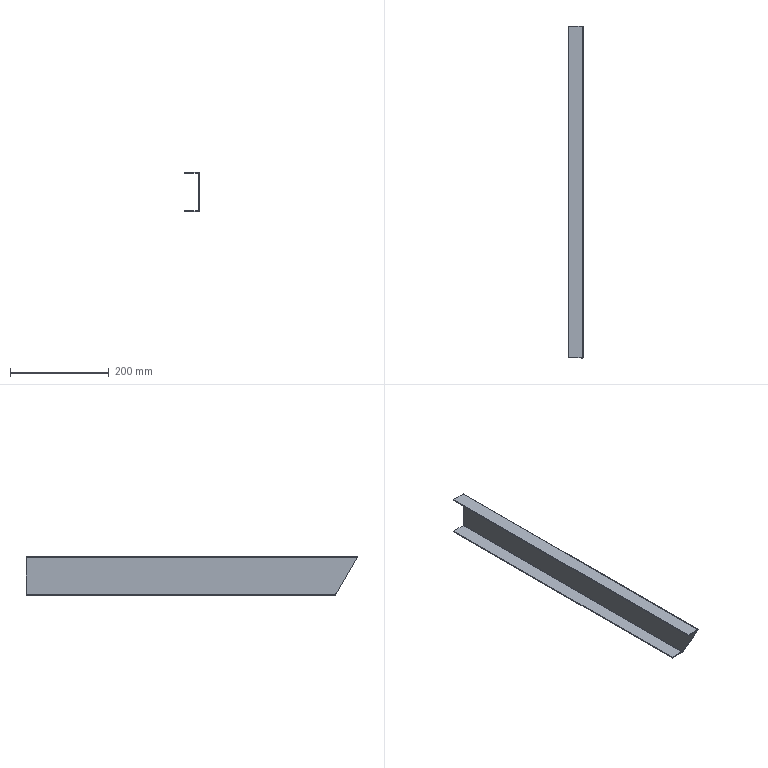Part | STEP file | Guard Rib | 1 solid | 19 faces | box 30 x 673.333 x 80 mm | volume 175185 mm3 | plane 13 | cylinder 5 | spline 1 | commonest cylinder face diameters 1 x3 5 x2
STEP:
#1=CARTESIAN_POINT('',(0.,265.398,-132.691));
#2=VERTEX_POINT('',#1);
#3=CARTESIAN_POINT('',(0.,221.653,-56.923));
#4=VERTEX_POINT('',#3);
#5=CARTESIAN_POINT('',(0.,265.398,-132.691));
#6=DIRECTION('',(0.,-0.5,0.866));
#7=VECTOR('',#6,1000.);
#8=LINE('',#5,#7);
#9=EDGE_CURVE('',#2,#4,#8,.T.);
#10=ORIENTED_EDGE('',*,*,#9,.F.);
#11=CARTESIAN_POINT('',(0.,265.398,-130.923));
#12=VERTEX_POINT('',#11);
#13=CARTESIAN_POINT('',(0.,265.398,0.));
#14=DIRECTION('',(0.,0.,-1.));
#15=VECTOR('',#14,1000.);
#16=LINE('',#13,#15);
#17=EDGE_CURVE('',#12,#2,#16,.T.);
#18=ORIENTED_EDGE('',*,*,#17,.F.);
#19=CARTESIAN_POINT('',(0.,266.398,-130.923));
#20=VERTEX_POINT('',#19);
#21=CARTESIAN_POINT('',(0.,265.898,-130.923));
#22=DIRECTION('',(-1.,0.,0.));
#23=DIRECTION('',(0.,0.,-1.));
#24=AXIS2_PLACEMENT_3D('',#21,#22,#23);
#25=CIRCLE('',#24,0.5);
#26=EDGE_CURVE('',#12,#20,#25,.T.);
#27=ORIENTED_EDGE('',*,*,#26,.T.);
#28=CARTESIAN_POINT('',(0.,266.398,-131.923));
#29=VERTEX_POINT('',#28);
#30=CARTESIAN_POINT('',(0.,266.398,-130.923));
#31=DIRECTION('',(0.,0.,1.));
#32=VECTOR('',#31,1000.);
#33=LINE('',#30,#32);
#34=EDGE_CURVE('',#29,#20,#33,.T.);
#35=ORIENTED_EDGE('',*,*,#34,.F.);
#36=CARTESIAN_POINT('',(0.,893.543,-131.923));
#37=VERTEX_POINT('',#36);
#38=CARTESIAN_POINT('',(0.,0.,-131.923));
#39=DIRECTION('',(0.,-1.,0.));
#40=VECTOR('',#39,1000.);
#41=LINE('',#38,#40);
#42=EDGE_CURVE('',#37,#29,#41,.T.);
#43=ORIENTED_EDGE('',*,*,#42,.F.);
#44=CARTESIAN_POINT('',(0.,893.543,-56.923));
#45=VERTEX_POINT('',#44);
#46=CARTESIAN_POINT('',(0.,893.543,0.));
#47=DIRECTION('',(0.,0.,-1.));
#48=VECTOR('',#47,1000.);
#49=LINE('',#46,#48);
#50=EDGE_CURVE('',#45,#37,#49,.T.);
#51=ORIENTED_EDGE('',*,*,#50,.F.);
#52=CARTESIAN_POINT('',(0.,0.,-56.923));
#53=DIRECTION('',(0.,1.,0.));
#54=VECTOR('',#53,1000.);
#55=LINE('',#52,#54);
#56=EDGE_CURVE('',#4,#45,#55,.T.);
#57=ORIENTED_EDGE('',*,*,#56,.F.);
#58=EDGE_LOOP('',(#10,#18,#27,#35,#43,#51,#57));
#59=FACE_OUTER_BOUND('',#58,.T.);
#60=CARTESIAN_POINT('',(0.,0.,0.));
#61=DIRECTION('',(-1.,0.,0.));
#62=DIRECTION('',(0.,0.,1.));
#63=AXIS2_PLACEMENT_3D('',#60,#61,#62);
#64=PLANE('',#63);
#65=ADVANCED_FACE('',(#59),#64,.F.);
#66=CARTESIAN_POINT('',(-2.5,893.543,-54.423));
#67=VERTEX_POINT('',#66);
#68=CARTESIAN_POINT('',(-2.5,220.21,-54.423));
#69=VERTEX_POINT('',#68);
#70=CARTESIAN_POINT('',(-2.5,893.543,-54.423));
#71=DIRECTION('',(0.,-1.,0.));
#72=VECTOR('',#71,1000.);
#73=LINE('',#70,#72);
#74=EDGE_CURVE('',#67,#69,#73,.T.);
#75=ORIENTED_EDGE('',*,*,#74,.T.);
#76=CARTESIAN_POINT('',(-2.5,220.21,-54.423));
#77=CARTESIAN_POINT('',(-2.17,220.332,-54.423));
#78=CARTESIAN_POINT('',(-1.85,220.449,-54.487));
#79=CARTESIAN_POINT('',(-1.393,220.631,-54.676));
#80=CARTESIAN_POINT('',(-1.248,220.691,-54.753));
#81=CARTESIAN_POINT('',(-0.9774,220.81,-54.934));
#82=CARTESIAN_POINT('',(-0.8497,220.871,-55.038));
#83=CARTESIAN_POINT('',(-0.6169,220.992,-55.271));
#84=CARTESIAN_POINT('',(-0.5135,221.051,-55.397));
#85=CARTESIAN_POINT('',(-0.3321,221.171,-55.668));
#86=CARTESIAN_POINT('',(-0.2536,221.232,-55.814));
#87=CARTESIAN_POINT('',(-0.128,221.352,-56.117));
#88=CARTESIAN_POINT('',(-0.08064,221.412,-56.273));
#89=CARTESIAN_POINT('',(-0.01656,221.532,-56.593));
#90=CARTESIAN_POINT('',(0.,221.593,-56.758));
#91=CARTESIAN_POINT('',(0.,221.653,-56.923));
#92=B_SPLINE_CURVE_WITH_KNOTS('',3,(#76,#77,#78,#79,#80,#81,#82,#83,#84,#85,#86,#87,#88,#89,#90,#91),.UNSPECIFIED.,.F.,.F.,(4,2,2,2,2,2,2,4),(0.,0.001038,0.001557,0.002076,0.002595,0.003114,0.003633,0.004151),.UNSPECIFIED.);
#93=EDGE_CURVE('',#69,#4,#92,.T.);
#94=ORIENTED_EDGE('',*,*,#93,.T.);
#95=ORIENTED_EDGE('',*,*,#56,.T.);
#96=CARTESIAN_POINT('',(-2.5,893.543,-56.923));
#97=DIRECTION('',(0.,-1.,0.));
#98=DIRECTION('',(0.,0.,1.));
#99=AXIS2_PLACEMENT_3D('',#96,#97,#98);
#100=CIRCLE('',#99,2.5);
#101=EDGE_CURVE('',#45,#67,#100,.T.);
#102=ORIENTED_EDGE('',*,*,#101,.T.);
#103=EDGE_LOOP('',(#75,#94,#95,#102));
#104=FACE_OUTER_BOUND('',#103,.T.);
#105=CARTESIAN_POINT('',(-2.5,893.543,-56.923));
#106=DIRECTION('',(0.,1.,0.));
#107=DIRECTION('',(0.,0.,1.));
#108=AXIS2_PLACEMENT_3D('',#105,#106,#107);
#109=CYLINDRICAL_SURFACE('',#108,2.5);
#110=ADVANCED_FACE('',(#104),#109,.T.);
#111=CARTESIAN_POINT('',(-2.,221.653,-56.923));
#112=VERTEX_POINT('',#111);
#113=CARTESIAN_POINT('',(-2.,265.398,-132.691));
#114=VERTEX_POINT('',#113);
#115=CARTESIAN_POINT('',(-2.,220.21,-54.423));
#116=DIRECTION('',(0.,0.5,-0.866));
#117=VECTOR('',#116,1000.);
#118=LINE('',#115,#117);
#119=EDGE_CURVE('',#112,#114,#118,.T.);
#120=ORIENTED_EDGE('',*,*,#119,.T.);
#121=CARTESIAN_POINT('',(-2.,265.398,-132.691));
#122=DIRECTION('',(1.,0.,0.));
#123=VECTOR('',#122,1000.);
#124=LINE('',#121,#123);
#125=EDGE_CURVE('',#114,#2,#124,.T.);
#126=ORIENTED_EDGE('',*,*,#125,.T.);
#127=ORIENTED_EDGE('',*,*,#9,.T.);
#128=CARTESIAN_POINT('',(-2.,221.653,-56.923));
#129=DIRECTION('',(-1.,0.,0.));
#130=VECTOR('',#129,1000.);
#131=LINE('',#128,#130);
#132=EDGE_CURVE('',#4,#112,#131,.T.);
#133=ORIENTED_EDGE('',*,*,#132,.T.);
#134=EDGE_LOOP('',(#120,#126,#127,#133));
#135=FACE_OUTER_BOUND('',#134,.T.);
#136=CARTESIAN_POINT('',(-2.,220.21,-54.423));
#137=DIRECTION('',(0.,-0.866,-0.5));
#138=DIRECTION('',(0.,0.5,-0.866));
#139=AXIS2_PLACEMENT_3D('',#136,#137,#138);
#140=PLANE('',#139);
#141=ADVANCED_FACE('',(#135),#140,.T.);
#142=ORIENTED_EDGE('',*,*,#125,.F.);
#143=CARTESIAN_POINT('',(-2.,265.398,-130.923));
#144=VERTEX_POINT('',#143);
#145=CARTESIAN_POINT('',(-2.,265.398,-132.691));
#146=DIRECTION('',(0.,0.,1.));
#147=VECTOR('',#146,1000.);
#148=LINE('',#145,#147);
#149=EDGE_CURVE('',#114,#144,#148,.T.);
#150=ORIENTED_EDGE('',*,*,#149,.T.);
#151=CARTESIAN_POINT('',(-2.,265.398,-130.923));
#152=DIRECTION('',(1.,0.,0.));
#153=VECTOR('',#152,1000.);
#154=LINE('',#151,#153);
#155=EDGE_CURVE('',#144,#12,#154,.T.);
#156=ORIENTED_EDGE('',*,*,#155,.T.);
#157=ORIENTED_EDGE('',*,*,#17,.T.);
#158=EDGE_LOOP('',(#142,#150,#156,#157));
#159=FACE_OUTER_BOUND('',#158,.T.);
#160=CARTESIAN_POINT('',(-2.,265.398,-132.691));
#161=DIRECTION('',(0.,1.,0.));
#162=DIRECTION('',(0.,0.,1.));
#163=AXIS2_PLACEMENT_3D('',#160,#161,#162);
#164=PLANE('',#163);
#165=ADVANCED_FACE('',(#159),#164,.T.);
#166=CARTESIAN_POINT('',(-2.5,266.398,-134.423));
#167=VERTEX_POINT('',#166);
#168=CARTESIAN_POINT('',(-2.5,893.543,-134.423));
#169=VERTEX_POINT('',#168);
#170=CARTESIAN_POINT('',(-2.5,266.398,-134.423));
#171=DIRECTION('',(0.,1.,0.));
#172=VECTOR('',#171,1000.);
#173=LINE('',#170,#172);
#174=EDGE_CURVE('',#167,#169,#173,.T.);
#175=ORIENTED_EDGE('',*,*,#174,.T.);
#176=CARTESIAN_POINT('',(-2.5,893.543,-131.923));
#177=DIRECTION('',(0.,-1.,0.));
#178=DIRECTION('',(0.,0.,-1.));
#179=AXIS2_PLACEMENT_3D('',#176,#177,#178);
#180=CIRCLE('',#179,2.5);
#181=EDGE_CURVE('',#169,#37,#180,.T.);
#182=ORIENTED_EDGE('',*,*,#181,.T.);
#183=ORIENTED_EDGE('',*,*,#42,.T.);
#184=CARTESIAN_POINT('',(-2.5,266.398,-131.923));
#185=DIRECTION('',(0.,1.,0.));
#186=DIRECTION('',(0.,0.,-1.));
#187=AXIS2_PLACEMENT_3D('',#184,#185,#186);
#188=CIRCLE('',#187,2.5);
#189=EDGE_CURVE('',#29,#167,#188,.T.);
#190=ORIENTED_EDGE('',*,*,#189,.T.);
#191=EDGE_LOOP('',(#175,#182,#183,#190));
#192=FACE_OUTER_BOUND('',#191,.T.);
#193=CARTESIAN_POINT('',(-2.5,266.398,-131.923));
#194=DIRECTION('',(0.,-1.,0.));
#195=DIRECTION('',(0.,0.,-1.));
#196=AXIS2_PLACEMENT_3D('',#193,#194,#195);
#197=CYLINDRICAL_SURFACE('',#196,2.5);
#198=ADVANCED_FACE('',(#192),#197,.T.);
#199=ORIENTED_EDGE('',*,*,#50,.T.);
#200=ORIENTED_EDGE('',*,*,#181,.F.);
#201=CARTESIAN_POINT('',(-30.,893.543,-134.423));
#202=VERTEX_POINT('',#201);
#203=CARTESIAN_POINT('',(0.,893.543,-134.423));
#204=DIRECTION('',(1.,0.,0.));
#205=VECTOR('',#204,1000.);
#206=LINE('',#203,#205);
#207=EDGE_CURVE('',#202,#169,#206,.T.);
#208=ORIENTED_EDGE('',*,*,#207,.F.);
#209=CARTESIAN_POINT('',(-30.,893.543,-132.423));
#210=VERTEX_POINT('',#209);
#211=CARTESIAN_POINT('',(-30.,893.543,-134.423));
#212=DIRECTION('',(0.,0.,1.));
#213=VECTOR('',#212,1000.);
#214=LINE('',#211,#213);
#215=EDGE_CURVE('',#202,#210,#214,.T.);
#216=ORIENTED_EDGE('',*,*,#215,.T.);
#217=CARTESIAN_POINT('',(-2.5,893.543,-132.423));
#218=VERTEX_POINT('',#217);
#219=CARTESIAN_POINT('',(-30.,893.543,-132.423));
#220=DIRECTION('',(1.,0.,0.));
#221=VECTOR('',#220,1000.);
#222=LINE('',#219,#221);
#223=EDGE_CURVE('',#210,#218,#222,.T.);
#224=ORIENTED_EDGE('',*,*,#223,.T.);
#225=CARTESIAN_POINT('',(-2.,893.543,-131.923));
#226=VERTEX_POINT('',#225);
#227=CARTESIAN_POINT('',(-2.5,893.543,-131.923));
#228=DIRECTION('',(0.,-1.,0.));
#229=DIRECTION('',(0.,0.,-1.));
#230=AXIS2_PLACEMENT_3D('',#227,#228,#229);
#231=CIRCLE('',#230,0.5);
#232=EDGE_CURVE('',#218,#226,#231,.T.);
#233=ORIENTED_EDGE('',*,*,#232,.T.);
#234=CARTESIAN_POINT('',(-2.,893.543,-56.923));
#235=VERTEX_POINT('',#234);
#236=CARTESIAN_POINT('',(-2.,893.543,-54.423));
#237=DIRECTION('',(0.,0.,1.));
#238=VECTOR('',#237,1000.);
#239=LINE('',#236,#238);
#240=EDGE_CURVE('',#226,#235,#239,.T.);
#241=ORIENTED_EDGE('',*,*,#240,.T.);
#242=CARTESIAN_POINT('',(-2.5,893.543,-56.423));
#243=VERTEX_POINT('',#242);
#244=CARTESIAN_POINT('',(-2.5,893.543,-56.923));
#245=DIRECTION('',(0.,-1.,0.));
#246=DIRECTION('',(0.,0.,1.));
#247=AXIS2_PLACEMENT_3D('',#244,#245,#246);
#248=CIRCLE('',#247,0.5);
#249=EDGE_CURVE('',#235,#243,#248,.T.);
#250=ORIENTED_EDGE('',*,*,#249,.T.);
#251=CARTESIAN_POINT('',(-30.,893.543,-56.423));
#252=VERTEX_POINT('',#251);
#253=CARTESIAN_POINT('',(-30.,893.543,-56.423));
#254=DIRECTION('',(-1.,0.,0.));
#255=VECTOR('',#254,1000.);
#256=LINE('',#253,#255);
#257=EDGE_CURVE('',#243,#252,#256,.T.);
#258=ORIENTED_EDGE('',*,*,#257,.T.);
#259=CARTESIAN_POINT('',(-30.,893.543,-54.423));
#260=VERTEX_POINT('',#259);
#261=CARTESIAN_POINT('',(-30.,893.543,-54.423));
#262=DIRECTION('',(0.,0.,1.));
#263=VECTOR('',#262,1000.);
#264=LINE('',#261,#263);
#265=EDGE_CURVE('',#252,#260,#264,.T.);
#266=ORIENTED_EDGE('',*,*,#265,.T.);
#267=CARTESIAN_POINT('',(0.,893.543,-54.423));
#268=DIRECTION('',(1.,0.,0.));
#269=VECTOR('',#268,1000.);
#270=LINE('',#267,#269);
#271=EDGE_CURVE('',#260,#67,#270,.T.);
#272=ORIENTED_EDGE('',*,*,#271,.T.);
#273=ORIENTED_EDGE('',*,*,#101,.F.);
#274=EDGE_LOOP('',(#199,#200,#208,#216,#224,#233,#241,#250,#258,#266,#272,#273));
#275=FACE_OUTER_BOUND('',#274,.T.);
#276=CARTESIAN_POINT('',(-2.,893.543,-54.423));
#277=DIRECTION('',(0.,1.,0.));
#278=DIRECTION('',(0.,0.,1.));
#279=AXIS2_PLACEMENT_3D('',#276,#277,#278);
#280=PLANE('',#279);
#281=ADVANCED_FACE('',(#275),#280,.T.);
#282=CARTESIAN_POINT('',(-2.5,220.21,-56.423));
#283=VERTEX_POINT('',#282);
#284=CARTESIAN_POINT('',(-2.5,220.21,-56.423));
#285=CARTESIAN_POINT('',(-2.434,220.331,-56.423));
#286=CARTESIAN_POINT('',(-2.369,220.451,-56.436));
#287=CARTESIAN_POINT('',(-2.249,220.69,-56.486));
#288=CARTESIAN_POINT('',(-2.193,220.811,-56.523));
#289=CARTESIAN_POINT('',(-2.054,221.173,-56.662));
#290=CARTESIAN_POINT('',(-2.,221.411,-56.791));
#291=CARTESIAN_POINT('',(-2.,221.653,-56.923));
#292=B_SPLINE_CURVE_WITH_KNOTS('',3,(#284,#285,#286,#287,#288,#289,#290,#291),.UNSPECIFIED.,.F.,.F.,(4,2,2,4),(0.,0.0004085,0.0008171,0.001634),.UNSPECIFIED.);
#293=EDGE_CURVE('',#283,#112,#292,.T.);
#294=ORIENTED_EDGE('',*,*,#293,.T.);
#295=ORIENTED_EDGE('',*,*,#132,.F.);
#296=ORIENTED_EDGE('',*,*,#93,.F.);
#297=CARTESIAN_POINT('',(-2.5,220.21,-55.423));
#298=DIRECTION('',(0.,0.,1.));
#299=VECTOR('',#298,1000.);
#300=LINE('',#297,#299);
#301=EDGE_CURVE('',#283,#69,#300,.T.);
#302=ORIENTED_EDGE('',*,*,#301,.F.);
#303=EDGE_LOOP('',(#294,#295,#296,#302));
#304=FACE_OUTER_BOUND('',#303,.T.);
#305=CARTESIAN_POINT('',(0.02,221.653,-56.923));
#306=CARTESIAN_POINT('',(0.02,221.533,-56.593));
#307=CARTESIAN_POINT('',(-0.04559,221.413,-56.264));
#308=CARTESIAN_POINT('',(-0.2981,221.172,-55.654));
#309=CARTESIAN_POINT('',(-0.4848,221.052,-55.375));
#310=CARTESIAN_POINT('',(-0.9513,220.812,-54.908));
#311=CARTESIAN_POINT('',(-1.231,220.691,-54.721));
#312=CARTESIAN_POINT('',(-1.84,220.451,-54.469));
#313=CARTESIAN_POINT('',(-2.17,220.33,-54.403));
#314=CARTESIAN_POINT('',(-2.5,220.21,-54.403));
#315=CARTESIAN_POINT('',(0.,221.653,-56.923));
#316=CARTESIAN_POINT('',(0.,221.533,-56.596));
#317=CARTESIAN_POINT('',(-0.06507,221.413,-56.269));
#318=CARTESIAN_POINT('',(-0.3155,221.172,-55.664));
#319=CARTESIAN_POINT('',(-0.5008,221.052,-55.387));
#320=CARTESIAN_POINT('',(-0.9636,220.812,-54.924));
#321=CARTESIAN_POINT('',(-1.241,220.691,-54.739));
#322=CARTESIAN_POINT('',(-1.846,220.451,-54.488));
#323=CARTESIAN_POINT('',(-2.173,220.33,-54.423));
#324=CARTESIAN_POINT('',(-2.5,220.21,-54.423));
#325=CARTESIAN_POINT('',(-2.,221.653,-56.923));
#326=CARTESIAN_POINT('',(-2.,221.533,-56.858));
#327=CARTESIAN_POINT('',(-2.013,221.413,-56.792));
#328=CARTESIAN_POINT('',(-2.063,221.172,-56.671));
#329=CARTESIAN_POINT('',(-2.1,221.052,-56.616));
#330=CARTESIAN_POINT('',(-2.193,220.812,-56.523));
#331=CARTESIAN_POINT('',(-2.248,220.691,-56.486));
#332=CARTESIAN_POINT('',(-2.369,220.451,-56.436));
#333=CARTESIAN_POINT('',(-2.435,220.33,-56.423));
#334=CARTESIAN_POINT('',(-2.5,220.21,-56.423));
#335=CARTESIAN_POINT('',(-2.02,221.653,-56.923));
#336=CARTESIAN_POINT('',(-2.02,221.533,-56.86));
#337=CARTESIAN_POINT('',(-2.033,221.413,-56.798));
#338=CARTESIAN_POINT('',(-2.081,221.172,-56.682));
#339=CARTESIAN_POINT('',(-2.116,221.052,-56.628));
#340=CARTESIAN_POINT('',(-2.205,220.812,-56.54));
#341=CARTESIAN_POINT('',(-2.258,220.691,-56.504));
#342=CARTESIAN_POINT('',(-2.374,220.451,-56.456));
#343=CARTESIAN_POINT('',(-2.437,220.33,-56.443));
#344=CARTESIAN_POINT('',(-2.5,220.21,-56.443));
#345=B_SPLINE_SURFACE_WITH_KNOTS('',1,3,((#305,#306,#307,#308,#309,#310,#311,#312,#313,#314),(#315,#316,#317,#318,#319,#320,#321,#322,#323,#324),(#325,#326,#327,#328,#329,#330,#331,#332,#333,#334),(#335,#336,#337,#338,#339,#340,#341,#342,#343,#344)),.UNSPECIFIED.,.F.,.F.,.F.,(2,1,1,2),(4,2,2,2,4),(-0.01,0.,1.,1.01),(0.,0.25,0.5,0.75,1.),.UNSPECIFIED.);
#346=ADVANCED_FACE('',(#304),#345,.F.);
#347=ORIENTED_EDGE('',*,*,#271,.F.);
#348=CARTESIAN_POINT('',(-30.,220.21,-54.423));
#349=VERTEX_POINT('',#348);
#350=CARTESIAN_POINT('',(-30.,0.,-54.423));
#351=DIRECTION('',(0.,1.,0.));
#352=VECTOR('',#351,1000.);
#353=LINE('',#350,#352);
#354=EDGE_CURVE('',#349,#260,#353,.T.);
#355=ORIENTED_EDGE('',*,*,#354,.F.);
#356=CARTESIAN_POINT('',(0.,220.21,-54.423));
#357=DIRECTION('',(-1.,0.,0.));
#358=VECTOR('',#357,1000.);
#359=LINE('',#356,#358);
#360=EDGE_CURVE('',#69,#349,#359,.T.);
#361=ORIENTED_EDGE('',*,*,#360,.F.);
#362=ORIENTED_EDGE('',*,*,#74,.F.);
#363=EDGE_LOOP('',(#347,#355,#361,#362));
#364=FACE_OUTER_BOUND('',#363,.T.);
#365=CARTESIAN_POINT('',(0.,0.,-54.423));
#366=DIRECTION('',(0.,0.,-1.));
#367=DIRECTION('',(-1.,0.,0.));
#368=AXIS2_PLACEMENT_3D('',#365,#366,#367);
#369=PLANE('',#368);
#370=ADVANCED_FACE('',(#364),#369,.F.);
#371=CARTESIAN_POINT('',(-2.,266.398,-130.923));
#372=VERTEX_POINT('',#371);
#373=CARTESIAN_POINT('',(-2.,265.898,-130.923));
#374=DIRECTION('',(1.,0.,0.));
#375=DIRECTION('',(0.,0.,-1.));
#376=AXIS2_PLACEMENT_3D('',#373,#374,#375);
#377=CIRCLE('',#376,0.5);
#378=EDGE_CURVE('',#372,#144,#377,.T.);
#379=ORIENTED_EDGE('',*,*,#378,.T.);
#380=ORIENTED_EDGE('',*,*,#149,.F.);
#381=ORIENTED_EDGE('',*,*,#119,.F.);
#382=CARTESIAN_POINT('',(-2.,0.,-56.923));
#383=DIRECTION('',(0.,1.,0.));
#384=VECTOR('',#383,1000.);
#385=LINE('',#382,#384);
#386=EDGE_CURVE('',#112,#235,#385,.T.);
#387=ORIENTED_EDGE('',*,*,#386,.T.);
#388=ORIENTED_EDGE('',*,*,#240,.F.);
#389=CARTESIAN_POINT('',(-2.,266.398,-131.923));
#390=VERTEX_POINT('',#389);
#391=CARTESIAN_POINT('',(-2.,0.,-131.923));
#392=DIRECTION('',(0.,-1.,0.));
#393=VECTOR('',#392,1000.);
#394=LINE('',#391,#393);
#395=EDGE_CURVE('',#226,#390,#394,.T.);
#396=ORIENTED_EDGE('',*,*,#395,.T.);
#397=CARTESIAN_POINT('',(-2.,266.398,-130.923));
#398=DIRECTION('',(0.,0.,-1.));
#399=VECTOR('',#398,1000.);
#400=LINE('',#397,#399);
#401=EDGE_CURVE('',#372,#390,#400,.T.);
#402=ORIENTED_EDGE('',*,*,#401,.F.);
#403=EDGE_LOOP('',(#379,#380,#381,#387,#388,#396,#402));
#404=FACE_OUTER_BOUND('',#403,.T.);
#405=CARTESIAN_POINT('',(-2.,0.,0.));
#406=DIRECTION('',(-1.,0.,0.));
#407=DIRECTION('',(0.,0.,1.));
#408=AXIS2_PLACEMENT_3D('',#405,#406,#407);
#409=PLANE('',#408);
#410=ADVANCED_FACE('',(#404),#409,.T.);
#411=ORIENTED_EDGE('',*,*,#26,.F.);
#412=ORIENTED_EDGE('',*,*,#155,.F.);
#413=ORIENTED_EDGE('',*,*,#378,.F.);
#414=CARTESIAN_POINT('',(-2.,266.398,-130.923));
#415=DIRECTION('',(-1.,0.,0.));
#416=VECTOR('',#415,1000.);
#417=LINE('',#414,#416);
#418=EDGE_CURVE('',#20,#372,#417,.T.);
#419=ORIENTED_EDGE('',*,*,#418,.F.);
#420=EDGE_LOOP('',(#411,#412,#413,#419));
#421=FACE_OUTER_BOUND('',#420,.T.);
#422=CARTESIAN_POINT('',(-2.,265.898,-130.923));
#423=DIRECTION('',(1.,0.,0.));
#424=DIRECTION('',(0.,0.,-1.));
#425=AXIS2_PLACEMENT_3D('',#422,#423,#424);
#426=CYLINDRICAL_SURFACE('',#425,0.5);
#427=ADVANCED_FACE('',(#421),#426,.F.);
#428=CARTESIAN_POINT('',(-30.,266.398,-134.423));
#429=VERTEX_POINT('',#428);
#430=CARTESIAN_POINT('',(0.,266.398,-134.423));
#431=DIRECTION('',(-1.,0.,0.));
#432=VECTOR('',#431,1000.);
#433=LINE('',#430,#432);
#434=EDGE_CURVE('',#167,#429,#433,.T.);
#435=ORIENTED_EDGE('',*,*,#434,.T.);
#436=CARTESIAN_POINT('',(-30.,0.,-134.423));
#437=DIRECTION('',(0.,1.,0.));
#438=VECTOR('',#437,1000.);
#439=LINE('',#436,#438);
#440=EDGE_CURVE('',#429,#202,#439,.T.);
#441=ORIENTED_EDGE('',*,*,#440,.T.);
#442=ORIENTED_EDGE('',*,*,#207,.T.);
#443=ORIENTED_EDGE('',*,*,#174,.F.);
#444=EDGE_LOOP('',(#435,#441,#442,#443));
#445=FACE_OUTER_BOUND('',#444,.T.);
#446=CARTESIAN_POINT('',(0.,0.,-134.423));
#447=DIRECTION('',(0.,0.,-1.));
#448=DIRECTION('',(-1.,0.,0.));
#449=AXIS2_PLACEMENT_3D('',#446,#447,#448);
#450=PLANE('',#449);
#451=ADVANCED_FACE('',(#445),#450,.T.);
#452=CARTESIAN_POINT('',(-2.5,266.398,-132.423));
#453=VERTEX_POINT('',#452);
#454=CARTESIAN_POINT('',(-2.5,266.398,-131.923));
#455=DIRECTION('',(0.,-1.,0.));
#456=DIRECTION('',(0.,0.,-1.));
#457=AXIS2_PLACEMENT_3D('',#454,#455,#456);
#458=CIRCLE('',#457,0.5);
#459=EDGE_CURVE('',#453,#390,#458,.T.);
#460=ORIENTED_EDGE('',*,*,#459,.F.);
#461=CARTESIAN_POINT('',(-30.,266.398,-132.423));
#462=VERTEX_POINT('',#461);
#463=CARTESIAN_POINT('',(-2.,266.398,-132.423));
#464=DIRECTION('',(-1.,0.,0.));
#465=VECTOR('',#464,1000.);
#466=LINE('',#463,#465);
#467=EDGE_CURVE('',#453,#462,#466,.T.);
#468=ORIENTED_EDGE('',*,*,#467,.T.);
#469=CARTESIAN_POINT('',(-30.,266.398,-134.423));
#470=DIRECTION('',(0.,0.,1.));
#471=VECTOR('',#470,1000.);
#472=LINE('',#469,#471);
#473=EDGE_CURVE('',#429,#462,#472,.T.);
#474=ORIENTED_EDGE('',*,*,#473,.F.);
#475=ORIENTED_EDGE('',*,*,#434,.F.);
#476=ORIENTED_EDGE('',*,*,#189,.F.);
#477=ORIENTED_EDGE('',*,*,#34,.T.);
#478=ORIENTED_EDGE('',*,*,#418,.T.);
#479=ORIENTED_EDGE('',*,*,#401,.T.);
#480=EDGE_LOOP('',(#460,#468,#474,#475,#476,#477,#478,#479));
#481=FACE_OUTER_BOUND('',#480,.T.);
#482=CARTESIAN_POINT('',(-2.5,266.398,-131.923));
#483=DIRECTION('',(0.,1.,0.));
#484=DIRECTION('',(0.,0.,1.));
#485=AXIS2_PLACEMENT_3D('',#482,#483,#484);
#486=PLANE('',#485);
#487=ADVANCED_FACE('',(#481),#486,.F.);
#488=ORIENTED_EDGE('',*,*,#360,.T.);
#489=CARTESIAN_POINT('',(-30.,220.21,-56.423));
#490=VERTEX_POINT('',#489);
#491=CARTESIAN_POINT('',(-30.,220.21,-54.423));
#492=DIRECTION('',(0.,0.,-1.));
#493=VECTOR('',#492,1000.);
#494=LINE('',#491,#493);
#495=EDGE_CURVE('',#349,#490,#494,.T.);
#496=ORIENTED_EDGE('',*,*,#495,.T.);
#497=CARTESIAN_POINT('',(-2.,220.21,-56.423));
#498=DIRECTION('',(1.,0.,0.));
#499=VECTOR('',#498,1000.);
#500=LINE('',#497,#499);
#501=EDGE_CURVE('',#490,#283,#500,.T.);
#502=ORIENTED_EDGE('',*,*,#501,.T.);
#503=ORIENTED_EDGE('',*,*,#301,.T.);
#504=EDGE_LOOP('',(#488,#496,#502,#503));
#505=FACE_OUTER_BOUND('',#504,.T.);
#506=CARTESIAN_POINT('',(-2.,220.21,-54.423));
#507=DIRECTION('',(0.,-1.,0.));
#508=DIRECTION('',(0.,0.,-1.));
#509=AXIS2_PLACEMENT_3D('',#506,#507,#508);
#510=PLANE('',#509);
#511=ADVANCED_FACE('',(#505),#510,.T.);
#512=ORIENTED_EDGE('',*,*,#354,.T.);
#513=ORIENTED_EDGE('',*,*,#265,.F.);
#514=CARTESIAN_POINT('',(-30.,220.21,-56.423));
#515=DIRECTION('',(0.,-1.,0.));
#516=VECTOR('',#515,1000.);
#517=LINE('',#514,#516);
#518=EDGE_CURVE('',#252,#490,#517,.T.);
#519=ORIENTED_EDGE('',*,*,#518,.T.);
#520=ORIENTED_EDGE('',*,*,#495,.F.);
#521=EDGE_LOOP('',(#512,#513,#519,#520));
#522=FACE_OUTER_BOUND('',#521,.T.);
#523=CARTESIAN_POINT('',(-30.,220.21,-54.423));
#524=DIRECTION('',(-1.,0.,0.));
#525=DIRECTION('',(0.,0.,1.));
#526=AXIS2_PLACEMENT_3D('',#523,#524,#525);
#527=PLANE('',#526);
#528=ADVANCED_FACE('',(#522),#527,.T.);
#529=ORIENTED_EDGE('',*,*,#232,.F.);
#530=CARTESIAN_POINT('',(-2.5,266.398,-132.423));
#531=DIRECTION('',(0.,1.,0.));
#532=VECTOR('',#531,1000.);
#533=LINE('',#530,#532);
#534=EDGE_CURVE('',#453,#218,#533,.T.);
#535=ORIENTED_EDGE('',*,*,#534,.F.);
#536=ORIENTED_EDGE('',*,*,#459,.T.);
#537=ORIENTED_EDGE('',*,*,#395,.F.);
#538=EDGE_LOOP('',(#529,#535,#536,#537));
#539=FACE_OUTER_BOUND('',#538,.T.);
#540=CARTESIAN_POINT('',(-2.5,266.398,-131.923));
#541=DIRECTION('',(0.,-1.,0.));
#542=DIRECTION('',(0.,0.,-1.));
#543=AXIS2_PLACEMENT_3D('',#540,#541,#542);
#544=CYLINDRICAL_SURFACE('',#543,0.5);
#545=ADVANCED_FACE('',(#539),#544,.F.);
#546=ORIENTED_EDGE('',*,*,#293,.F.);
#547=CARTESIAN_POINT('',(-2.5,893.543,-56.423));
#548=DIRECTION('',(0.,-1.,0.));
#549=VECTOR('',#548,1000.);
#550=LINE('',#547,#549);
#551=EDGE_CURVE('',#243,#283,#550,.T.);
#552=ORIENTED_EDGE('',*,*,#551,.F.);
#553=ORIENTED_EDGE('',*,*,#249,.F.);
#554=ORIENTED_EDGE('',*,*,#386,.F.);
#555=EDGE_LOOP('',(#546,#552,#553,#554));
#556=FACE_OUTER_BOUND('',#555,.T.);
#557=CARTESIAN_POINT('',(-2.5,893.543,-56.923));
#558=DIRECTION('',(0.,1.,0.));
#559=DIRECTION('',(0.,0.,1.));
#560=AXIS2_PLACEMENT_3D('',#557,#558,#559);
#561=CYLINDRICAL_SURFACE('',#560,0.5);
#562=ADVANCED_FACE('',(#556),#561,.F.);
#563=ORIENTED_EDGE('',*,*,#440,.F.);
#564=ORIENTED_EDGE('',*,*,#473,.T.);
#565=CARTESIAN_POINT('',(-30.,266.398,-132.423));
#566=DIRECTION('',(0.,1.,0.));
#567=VECTOR('',#566,1000.);
#568=LINE('',#565,#567);
#569=EDGE_CURVE('',#462,#210,#568,.T.);
#570=ORIENTED_EDGE('',*,*,#569,.T.);
#571=ORIENTED_EDGE('',*,*,#215,.F.);
#572=EDGE_LOOP('',(#563,#564,#570,#571));
#573=FACE_OUTER_BOUND('',#572,.T.);
#574=CARTESIAN_POINT('',(-30.,266.398,-134.423));
#575=DIRECTION('',(-1.,0.,0.));
#576=DIRECTION('',(0.,0.,1.));
#577=AXIS2_PLACEMENT_3D('',#574,#575,#576);
#578=PLANE('',#577);
#579=ADVANCED_FACE('',(#573),#578,.T.);
#580=ORIENTED_EDGE('',*,*,#501,.F.);
#581=ORIENTED_EDGE('',*,*,#518,.F.);
#582=ORIENTED_EDGE('',*,*,#257,.F.);
#583=ORIENTED_EDGE('',*,*,#551,.T.);
#584=EDGE_LOOP('',(#580,#581,#582,#583));
#585=FACE_OUTER_BOUND('',#584,.T.);
#586=CARTESIAN_POINT('',(0.,0.,-56.423));
#587=DIRECTION('',(0.,0.,-1.));
#588=DIRECTION('',(-1.,0.,0.));
#589=AXIS2_PLACEMENT_3D('',#586,#587,#588);
#590=PLANE('',#589);
#591=ADVANCED_FACE('',(#585),#590,.T.);
#592=ORIENTED_EDGE('',*,*,#223,.F.);
#593=ORIENTED_EDGE('',*,*,#569,.F.);
#594=ORIENTED_EDGE('',*,*,#467,.F.);
#595=ORIENTED_EDGE('',*,*,#534,.T.);
#596=EDGE_LOOP('',(#592,#593,#594,#595));
#597=FACE_OUTER_BOUND('',#596,.T.);
#598=CARTESIAN_POINT('',(0.,0.,-132.423));
#599=DIRECTION('',(0.,0.,-1.));
#600=DIRECTION('',(-1.,0.,0.));
#601=AXIS2_PLACEMENT_3D('',#598,#599,#600);
#602=PLANE('',#601);
#603=ADVANCED_FACE('',(#597),#602,.F.);
#604=CLOSED_SHELL('',(#65,#110,#141,#165,#198,#281,#346,#370,#410,#427,#451,#487,#511,#528,#545,#562,#579,#591,#603));
#605=MANIFOLD_SOLID_BREP('',#604);
#606=CARTESIAN_POINT('',(0.,0.,0.));
#607=DIRECTION('',(0.,0.,1.));
#608=DIRECTION('',(1.,0.,0.));
#609=AXIS2_PLACEMENT_3D('',#606,#607,#608);
#610=(LENGTH_UNIT()NAMED_UNIT(*)SI_UNIT(.MILLI.,.METRE.));
#611=UNCERTAINTY_MEASURE_WITH_UNIT(LENGTH_MEASURE(0.00001),#610,'','');
#612=(NAMED_UNIT(*)PLANE_ANGLE_UNIT()SI_UNIT($,.RADIAN.));
#613=(NAMED_UNIT(*)SI_UNIT($,.STERADIAN.)SOLID_ANGLE_UNIT());
#614=(GEOMETRIC_REPRESENTATION_CONTEXT(3)GLOBAL_UNCERTAINTY_ASSIGNED_CONTEXT((#611))GLOBAL_UNIT_ASSIGNED_CONTEXT((#610,#612,#613))REPRESENTATION_CONTEXT('',''));
#615=ADVANCED_BREP_SHAPE_REPRESENTATION('',(#605,#609),#614);